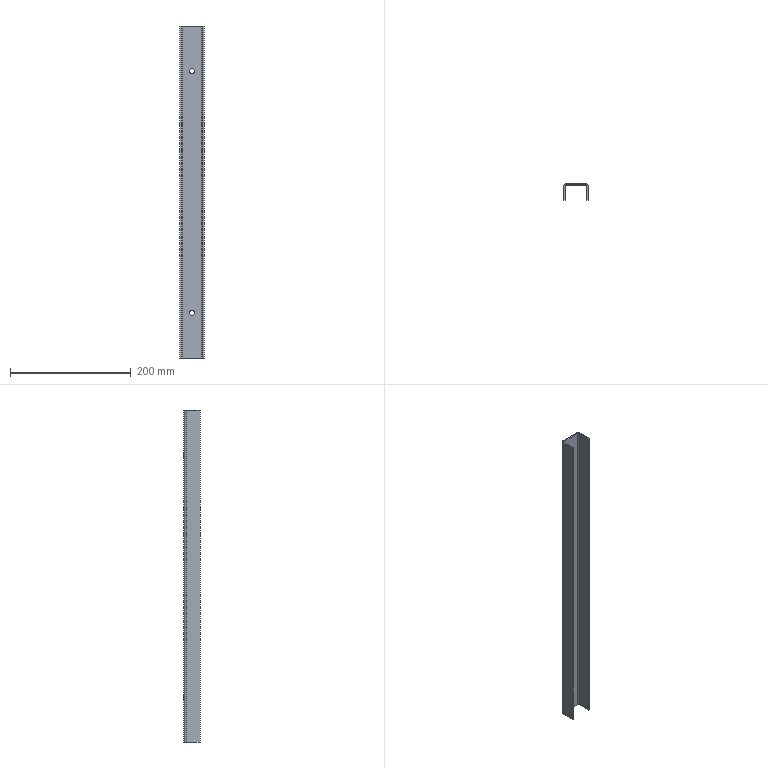Part | STEP file | SYL_0392D6J1SYL0380DJ10-1718718 | 1 solid | 26 faces | box 40 x 27 x 550 mm | volume 95966 mm3 | plane 18 | cylinder 8 | commonest cylinder face diameters 8 x6 4 x2
STEP:
#1=CARTESIAN_POINT('',(0.,14.5,196.));
#2=VERTEX_POINT('',#1);
#3=CARTESIAN_POINT('',(0.,12.5,196.));
#4=VERTEX_POINT('',#3);
#5=CARTESIAN_POINT('',(0.,12.5,196.));
#6=DIRECTION('',(0.,-1.,0.));
#7=VECTOR('',#6,1000.);
#8=LINE('',#5,#7);
#9=EDGE_CURVE('',#2,#4,#8,.T.);
#10=ORIENTED_EDGE('',*,*,#9,.F.);
#11=CARTESIAN_POINT('',(0.,14.5,204.));
#12=VERTEX_POINT('',#11);
#13=CARTESIAN_POINT('',(0.,14.5,200.));
#14=DIRECTION('',(0.,1.,0.));
#15=DIRECTION('',(0.,0.,1.));
#16=AXIS2_PLACEMENT_3D('',#13,#14,#15);
#17=CIRCLE('',#16,4.);
#18=EDGE_CURVE('',#2,#12,#17,.T.);
#19=ORIENTED_EDGE('',*,*,#18,.T.);
#20=CARTESIAN_POINT('',(0.,12.5,204.));
#21=VERTEX_POINT('',#20);
#22=CARTESIAN_POINT('',(0.,12.5,204.));
#23=DIRECTION('',(0.,-1.,0.));
#24=VECTOR('',#23,1000.);
#25=LINE('',#22,#24);
#26=EDGE_CURVE('',#12,#21,#25,.T.);
#27=ORIENTED_EDGE('',*,*,#26,.T.);
#28=CARTESIAN_POINT('',(0.,12.5,200.));
#29=DIRECTION('',(0.,1.,0.));
#30=DIRECTION('',(0.,0.,-1.));
#31=AXIS2_PLACEMENT_3D('',#28,#29,#30);
#32=CIRCLE('',#31,4.);
#33=EDGE_CURVE('',#4,#21,#32,.T.);
#34=ORIENTED_EDGE('',*,*,#33,.F.);
#35=EDGE_LOOP('',(#10,#19,#27,#34));
#36=FACE_OUTER_BOUND('',#35,.T.);
#37=CARTESIAN_POINT('',(0.,12.5,200.));
#38=DIRECTION('',(0.,-1.,0.));
#39=DIRECTION('',(0.,0.,-1.));
#40=AXIS2_PLACEMENT_3D('',#37,#38,#39);
#41=CYLINDRICAL_SURFACE('',#40,4.);
#42=ADVANCED_FACE('',(#36),#41,.F.);
#43=CARTESIAN_POINT('',(0.,14.5,-204.));
#44=VERTEX_POINT('',#43);
#45=CARTESIAN_POINT('',(0.,12.5,-204.));
#46=VERTEX_POINT('',#45);
#47=CARTESIAN_POINT('',(0.,12.5,-204.));
#48=DIRECTION('',(0.,-1.,0.));
#49=VECTOR('',#48,1000.);
#50=LINE('',#47,#49);
#51=EDGE_CURVE('',#44,#46,#50,.T.);
#52=ORIENTED_EDGE('',*,*,#51,.F.);
#53=CARTESIAN_POINT('',(0.,14.5,-196.));
#54=VERTEX_POINT('',#53);
#55=CARTESIAN_POINT('',(0.,14.5,-200.));
#56=DIRECTION('',(0.,1.,0.));
#57=DIRECTION('',(0.,0.,1.));
#58=AXIS2_PLACEMENT_3D('',#55,#56,#57);
#59=CIRCLE('',#58,4.);
#60=EDGE_CURVE('',#44,#54,#59,.T.);
#61=ORIENTED_EDGE('',*,*,#60,.T.);
#62=CARTESIAN_POINT('',(0.,12.5,-196.));
#63=VERTEX_POINT('',#62);
#64=CARTESIAN_POINT('',(0.,12.5,-196.));
#65=DIRECTION('',(0.,-1.,0.));
#66=VECTOR('',#65,1000.);
#67=LINE('',#64,#66);
#68=EDGE_CURVE('',#54,#63,#67,.T.);
#69=ORIENTED_EDGE('',*,*,#68,.T.);
#70=CARTESIAN_POINT('',(0.,12.5,-200.));
#71=DIRECTION('',(0.,1.,0.));
#72=DIRECTION('',(0.,0.,-1.));
#73=AXIS2_PLACEMENT_3D('',#70,#71,#72);
#74=CIRCLE('',#73,4.);
#75=EDGE_CURVE('',#46,#63,#74,.T.);
#76=ORIENTED_EDGE('',*,*,#75,.F.);
#77=EDGE_LOOP('',(#52,#61,#69,#76));
#78=FACE_OUTER_BOUND('',#77,.T.);
#79=CARTESIAN_POINT('',(0.,12.5,-200.));
#80=DIRECTION('',(0.,-1.,0.));
#81=DIRECTION('',(0.,0.,-1.));
#82=AXIS2_PLACEMENT_3D('',#79,#80,#81);
#83=CYLINDRICAL_SURFACE('',#82,4.);
#84=ADVANCED_FACE('',(#78),#83,.F.);
#85=CARTESIAN_POINT('',(16.,14.5,-275.));
#86=VERTEX_POINT('',#85);
#87=CARTESIAN_POINT('',(16.,12.5,-275.));
#88=VERTEX_POINT('',#87);
#89=CARTESIAN_POINT('',(16.,12.5,-275.));
#90=DIRECTION('',(0.,-1.,0.));
#91=VECTOR('',#90,1000.);
#92=LINE('',#89,#91);
#93=EDGE_CURVE('',#86,#88,#92,.T.);
#94=ORIENTED_EDGE('',*,*,#93,.F.);
#95=CARTESIAN_POINT('',(20.,10.5,-275.));
#96=VERTEX_POINT('',#95);
#97=CARTESIAN_POINT('',(16.,10.5,-275.));
#98=DIRECTION('',(0.,0.,1.));
#99=DIRECTION('',(1.,0.,0.));
#100=AXIS2_PLACEMENT_3D('',#97,#98,#99);
#101=CIRCLE('',#100,4.);
#102=EDGE_CURVE('',#96,#86,#101,.T.);
#103=ORIENTED_EDGE('',*,*,#102,.F.);
#104=CARTESIAN_POINT('',(18.,10.5,-275.));
#105=VERTEX_POINT('',#104);
#106=CARTESIAN_POINT('',(18.,10.5,-275.));
#107=DIRECTION('',(-1.,0.,0.));
#108=VECTOR('',#107,1000.);
#109=LINE('',#106,#108);
#110=EDGE_CURVE('',#96,#105,#109,.T.);
#111=ORIENTED_EDGE('',*,*,#110,.T.);
#112=CARTESIAN_POINT('',(16.,10.5,-275.));
#113=DIRECTION('',(0.,0.,1.));
#114=DIRECTION('',(1.,0.,0.));
#115=AXIS2_PLACEMENT_3D('',#112,#113,#114);
#116=CIRCLE('',#115,2.);
#117=EDGE_CURVE('',#105,#88,#116,.T.);
#118=ORIENTED_EDGE('',*,*,#117,.T.);
#119=EDGE_LOOP('',(#94,#103,#111,#118));
#120=FACE_OUTER_BOUND('',#119,.T.);
#121=CARTESIAN_POINT('',(16.,10.5,-275.));
#122=DIRECTION('',(0.,0.,-1.));
#123=DIRECTION('',(-1.,0.,0.));
#124=AXIS2_PLACEMENT_3D('',#121,#122,#123);
#125=PLANE('',#124);
#126=ADVANCED_FACE('',(#120),#125,.T.);
#127=ORIENTED_EDGE('',*,*,#110,.F.);
#128=CARTESIAN_POINT('',(20.,-12.5,-275.));
#129=VERTEX_POINT('',#128);
#130=CARTESIAN_POINT('',(20.,12.5,-275.));
#131=DIRECTION('',(0.,-1.,0.));
#132=VECTOR('',#131,1000.);
#133=LINE('',#130,#132);
#134=EDGE_CURVE('',#96,#129,#133,.T.);
#135=ORIENTED_EDGE('',*,*,#134,.T.);
#136=CARTESIAN_POINT('',(18.,-12.5,-275.));
#137=VERTEX_POINT('',#136);
#138=CARTESIAN_POINT('',(18.,-12.5,-275.));
#139=DIRECTION('',(-1.,0.,0.));
#140=VECTOR('',#139,1000.);
#141=LINE('',#138,#140);
#142=EDGE_CURVE('',#129,#137,#141,.T.);
#143=ORIENTED_EDGE('',*,*,#142,.T.);
#144=CARTESIAN_POINT('',(18.,10.5,-275.));
#145=DIRECTION('',(0.,-1.,0.));
#146=VECTOR('',#145,1000.);
#147=LINE('',#144,#146);
#148=EDGE_CURVE('',#105,#137,#147,.T.);
#149=ORIENTED_EDGE('',*,*,#148,.F.);
#150=EDGE_LOOP('',(#127,#135,#143,#149));
#151=FACE_OUTER_BOUND('',#150,.T.);
#152=CARTESIAN_POINT('',(18.,10.5,-275.));
#153=DIRECTION('',(0.,0.,-1.));
#154=DIRECTION('',(0.,-1.,0.));
#155=AXIS2_PLACEMENT_3D('',#152,#153,#154);
#156=PLANE('',#155);
#157=ADVANCED_FACE('',(#151),#156,.T.);
#158=ORIENTED_EDGE('',*,*,#142,.F.);
#159=CARTESIAN_POINT('',(20.,-12.5,275.));
#160=VERTEX_POINT('',#159);
#161=CARTESIAN_POINT('',(20.,-12.5,-275.));
#162=DIRECTION('',(0.,0.,1.));
#163=VECTOR('',#162,1000.);
#164=LINE('',#161,#163);
#165=EDGE_CURVE('',#129,#160,#164,.T.);
#166=ORIENTED_EDGE('',*,*,#165,.T.);
#167=CARTESIAN_POINT('',(18.,-12.5,275.));
#168=VERTEX_POINT('',#167);
#169=CARTESIAN_POINT('',(18.,-12.5,275.));
#170=DIRECTION('',(-1.,0.,0.));
#171=VECTOR('',#170,1000.);
#172=LINE('',#169,#171);
#173=EDGE_CURVE('',#160,#168,#172,.T.);
#174=ORIENTED_EDGE('',*,*,#173,.T.);
#175=CARTESIAN_POINT('',(18.,-12.5,-275.));
#176=DIRECTION('',(0.,0.,1.));
#177=VECTOR('',#176,1000.);
#178=LINE('',#175,#177);
#179=EDGE_CURVE('',#137,#168,#178,.T.);
#180=ORIENTED_EDGE('',*,*,#179,.F.);
#181=EDGE_LOOP('',(#158,#166,#174,#180));
#182=FACE_OUTER_BOUND('',#181,.T.);
#183=CARTESIAN_POINT('',(18.,-12.5,-275.));
#184=DIRECTION('',(0.,-1.,0.));
#185=DIRECTION('',(0.,0.,1.));
#186=AXIS2_PLACEMENT_3D('',#183,#184,#185);
#187=PLANE('',#186);
#188=ADVANCED_FACE('',(#182),#187,.T.);
#189=ORIENTED_EDGE('',*,*,#173,.F.);
#190=CARTESIAN_POINT('',(20.,10.5,275.));
#191=VERTEX_POINT('',#190);
#192=CARTESIAN_POINT('',(20.,12.5,275.));
#193=DIRECTION('',(0.,-1.,0.));
#194=VECTOR('',#193,1000.);
#195=LINE('',#192,#194);
#196=EDGE_CURVE('',#191,#160,#195,.T.);
#197=ORIENTED_EDGE('',*,*,#196,.F.);
#198=CARTESIAN_POINT('',(18.,10.5,275.));
#199=VERTEX_POINT('',#198);
#200=CARTESIAN_POINT('',(18.,10.5,275.));
#201=DIRECTION('',(-1.,0.,0.));
#202=VECTOR('',#201,1000.);
#203=LINE('',#200,#202);
#204=EDGE_CURVE('',#191,#199,#203,.T.);
#205=ORIENTED_EDGE('',*,*,#204,.T.);
#206=CARTESIAN_POINT('',(18.,10.5,275.));
#207=DIRECTION('',(0.,-1.,0.));
#208=VECTOR('',#207,1000.);
#209=LINE('',#206,#208);
#210=EDGE_CURVE('',#199,#168,#209,.T.);
#211=ORIENTED_EDGE('',*,*,#210,.T.);
#212=EDGE_LOOP('',(#189,#197,#205,#211));
#213=FACE_OUTER_BOUND('',#212,.T.);
#214=CARTESIAN_POINT('',(18.,10.5,275.));
#215=DIRECTION('',(0.,0.,-1.));
#216=DIRECTION('',(0.,-1.,0.));
#217=AXIS2_PLACEMENT_3D('',#214,#215,#216);
#218=PLANE('',#217);
#219=ADVANCED_FACE('',(#213),#218,.F.);
#220=ORIENTED_EDGE('',*,*,#204,.F.);
#221=CARTESIAN_POINT('',(16.,14.5,275.));
#222=VERTEX_POINT('',#221);
#223=CARTESIAN_POINT('',(16.,10.5,275.));
#224=DIRECTION('',(0.,0.,-1.));
#225=DIRECTION('',(1.,0.,0.));
#226=AXIS2_PLACEMENT_3D('',#223,#224,#225);
#227=CIRCLE('',#226,4.);
#228=EDGE_CURVE('',#222,#191,#227,.T.);
#229=ORIENTED_EDGE('',*,*,#228,.F.);
#230=CARTESIAN_POINT('',(16.,12.5,275.));
#231=VERTEX_POINT('',#230);
#232=CARTESIAN_POINT('',(16.,12.5,275.));
#233=DIRECTION('',(0.,-1.,0.));
#234=VECTOR('',#233,1000.);
#235=LINE('',#232,#234);
#236=EDGE_CURVE('',#222,#231,#235,.T.);
#237=ORIENTED_EDGE('',*,*,#236,.T.);
#238=CARTESIAN_POINT('',(16.,10.5,275.));
#239=DIRECTION('',(0.,0.,-1.));
#240=DIRECTION('',(0.,1.,0.));
#241=AXIS2_PLACEMENT_3D('',#238,#239,#240);
#242=CIRCLE('',#241,2.);
#243=EDGE_CURVE('',#231,#199,#242,.T.);
#244=ORIENTED_EDGE('',*,*,#243,.T.);
#245=EDGE_LOOP('',(#220,#229,#237,#244));
#246=FACE_OUTER_BOUND('',#245,.T.);
#247=CARTESIAN_POINT('',(16.,10.5,275.));
#248=DIRECTION('',(0.,0.,1.));
#249=DIRECTION('',(1.,0.,0.));
#250=AXIS2_PLACEMENT_3D('',#247,#248,#249);
#251=PLANE('',#250);
#252=ADVANCED_FACE('',(#246),#251,.T.);
#253=ORIENTED_EDGE('',*,*,#236,.F.);
#254=CARTESIAN_POINT('',(-16.,14.5,275.));
#255=VERTEX_POINT('',#254);
#256=CARTESIAN_POINT('',(-18.,14.5,275.));
#257=DIRECTION('',(1.,0.,0.));
#258=VECTOR('',#257,1000.);
#259=LINE('',#256,#258);
#260=EDGE_CURVE('',#255,#222,#259,.T.);
#261=ORIENTED_EDGE('',*,*,#260,.F.);
#262=CARTESIAN_POINT('',(-16.,12.5,275.));
#263=VERTEX_POINT('',#262);
#264=CARTESIAN_POINT('',(-16.,12.5,275.));
#265=DIRECTION('',(0.,-1.,0.));
#266=VECTOR('',#265,1000.);
#267=LINE('',#264,#266);
#268=EDGE_CURVE('',#255,#263,#267,.T.);
#269=ORIENTED_EDGE('',*,*,#268,.T.);
#270=CARTESIAN_POINT('',(-16.,12.5,275.));
#271=DIRECTION('',(1.,0.,0.));
#272=VECTOR('',#271,1000.);
#273=LINE('',#270,#272);
#274=EDGE_CURVE('',#263,#231,#273,.T.);
#275=ORIENTED_EDGE('',*,*,#274,.T.);
#276=EDGE_LOOP('',(#253,#261,#269,#275));
#277=FACE_OUTER_BOUND('',#276,.T.);
#278=CARTESIAN_POINT('',(-16.,12.5,275.));
#279=DIRECTION('',(0.,0.,-1.));
#280=DIRECTION('',(1.,0.,0.));
#281=AXIS2_PLACEMENT_3D('',#278,#279,#280);
#282=PLANE('',#281);
#283=ADVANCED_FACE('',(#277),#282,.F.);
#284=ORIENTED_EDGE('',*,*,#268,.F.);
#285=CARTESIAN_POINT('',(-20.,10.5,275.));
#286=VERTEX_POINT('',#285);
#287=CARTESIAN_POINT('',(-16.,10.5,275.));
#288=DIRECTION('',(0.,0.,-1.));
#289=DIRECTION('',(1.,0.,0.));
#290=AXIS2_PLACEMENT_3D('',#287,#288,#289);
#291=CIRCLE('',#290,4.);
#292=EDGE_CURVE('',#286,#255,#291,.T.);
#293=ORIENTED_EDGE('',*,*,#292,.F.);
#294=CARTESIAN_POINT('',(-18.,10.5,275.));
#295=VERTEX_POINT('',#294);
#296=CARTESIAN_POINT('',(-18.,10.5,275.));
#297=DIRECTION('',(1.,0.,0.));
#298=VECTOR('',#297,1000.);
#299=LINE('',#296,#298);
#300=EDGE_CURVE('',#286,#295,#299,.T.);
#301=ORIENTED_EDGE('',*,*,#300,.T.);
#302=CARTESIAN_POINT('',(-16.,10.5,275.));
#303=DIRECTION('',(0.,0.,-1.));
#304=DIRECTION('',(-1.,0.,0.));
#305=AXIS2_PLACEMENT_3D('',#302,#303,#304);
#306=CIRCLE('',#305,2.);
#307=EDGE_CURVE('',#295,#263,#306,.T.);
#308=ORIENTED_EDGE('',*,*,#307,.T.);
#309=EDGE_LOOP('',(#284,#293,#301,#308));
#310=FACE_OUTER_BOUND('',#309,.T.);
#311=CARTESIAN_POINT('',(-16.,10.5,275.));
#312=DIRECTION('',(0.,0.,1.));
#313=DIRECTION('',(1.,0.,0.));
#314=AXIS2_PLACEMENT_3D('',#311,#312,#313);
#315=PLANE('',#314);
#316=ADVANCED_FACE('',(#310),#315,.T.);
#317=ORIENTED_EDGE('',*,*,#300,.F.);
#318=CARTESIAN_POINT('',(-20.,-12.5,275.));
#319=VERTEX_POINT('',#318);
#320=CARTESIAN_POINT('',(-20.,-12.5,275.));
#321=DIRECTION('',(0.,1.,0.));
#322=VECTOR('',#321,1000.);
#323=LINE('',#320,#322);
#324=EDGE_CURVE('',#319,#286,#323,.T.);
#325=ORIENTED_EDGE('',*,*,#324,.F.);
#326=CARTESIAN_POINT('',(-18.,-12.5,275.));
#327=VERTEX_POINT('',#326);
#328=CARTESIAN_POINT('',(-18.,-12.5,275.));
#329=DIRECTION('',(1.,0.,0.));
#330=VECTOR('',#329,1000.);
#331=LINE('',#328,#330);
#332=EDGE_CURVE('',#319,#327,#331,.T.);
#333=ORIENTED_EDGE('',*,*,#332,.T.);
#334=CARTESIAN_POINT('',(-18.,-12.5,275.));
#335=DIRECTION('',(0.,1.,0.));
#336=VECTOR('',#335,1000.);
#337=LINE('',#334,#336);
#338=EDGE_CURVE('',#327,#295,#337,.T.);
#339=ORIENTED_EDGE('',*,*,#338,.T.);
#340=EDGE_LOOP('',(#317,#325,#333,#339));
#341=FACE_OUTER_BOUND('',#340,.T.);
#342=CARTESIAN_POINT('',(-18.,-12.5,275.));
#343=DIRECTION('',(0.,0.,-1.));
#344=DIRECTION('',(0.,1.,0.));
#345=AXIS2_PLACEMENT_3D('',#342,#343,#344);
#346=PLANE('',#345);
#347=ADVANCED_FACE('',(#341),#346,.F.);
#348=ORIENTED_EDGE('',*,*,#332,.F.);
#349=CARTESIAN_POINT('',(-20.,-12.5,-275.));
#350=VERTEX_POINT('',#349);
#351=CARTESIAN_POINT('',(-20.,-12.5,-275.));
#352=DIRECTION('',(0.,0.,1.));
#353=VECTOR('',#352,1000.);
#354=LINE('',#351,#353);
#355=EDGE_CURVE('',#350,#319,#354,.T.);
#356=ORIENTED_EDGE('',*,*,#355,.F.);
#357=CARTESIAN_POINT('',(-18.,-12.5,-275.));
#358=VERTEX_POINT('',#357);
#359=CARTESIAN_POINT('',(-18.,-12.5,-275.));
#360=DIRECTION('',(1.,0.,0.));
#361=VECTOR('',#360,1000.);
#362=LINE('',#359,#361);
#363=EDGE_CURVE('',#350,#358,#362,.T.);
#364=ORIENTED_EDGE('',*,*,#363,.T.);
#365=CARTESIAN_POINT('',(-18.,-12.5,-275.));
#366=DIRECTION('',(0.,0.,1.));
#367=VECTOR('',#366,1000.);
#368=LINE('',#365,#367);
#369=EDGE_CURVE('',#358,#327,#368,.T.);
#370=ORIENTED_EDGE('',*,*,#369,.T.);
#371=EDGE_LOOP('',(#348,#356,#364,#370));
#372=FACE_OUTER_BOUND('',#371,.T.);
#373=CARTESIAN_POINT('',(-18.,-12.5,-275.));
#374=DIRECTION('',(0.,1.,0.));
#375=DIRECTION('',(0.,0.,1.));
#376=AXIS2_PLACEMENT_3D('',#373,#374,#375);
#377=PLANE('',#376);
#378=ADVANCED_FACE('',(#372),#377,.F.);
#379=ORIENTED_EDGE('',*,*,#363,.F.);
#380=CARTESIAN_POINT('',(-20.,10.5,-275.));
#381=VERTEX_POINT('',#380);
#382=CARTESIAN_POINT('',(-20.,-12.5,-275.));
#383=DIRECTION('',(0.,1.,0.));
#384=VECTOR('',#383,1000.);
#385=LINE('',#382,#384);
#386=EDGE_CURVE('',#350,#381,#385,.T.);
#387=ORIENTED_EDGE('',*,*,#386,.T.);
#388=CARTESIAN_POINT('',(-18.,10.5,-275.));
#389=VERTEX_POINT('',#388);
#390=CARTESIAN_POINT('',(-18.,10.5,-275.));
#391=DIRECTION('',(1.,0.,0.));
#392=VECTOR('',#391,1000.);
#393=LINE('',#390,#392);
#394=EDGE_CURVE('',#381,#389,#393,.T.);
#395=ORIENTED_EDGE('',*,*,#394,.T.);
#396=CARTESIAN_POINT('',(-18.,-12.5,-275.));
#397=DIRECTION('',(0.,1.,0.));
#398=VECTOR('',#397,1000.);
#399=LINE('',#396,#398);
#400=EDGE_CURVE('',#358,#389,#399,.T.);
#401=ORIENTED_EDGE('',*,*,#400,.F.);
#402=EDGE_LOOP('',(#379,#387,#395,#401));
#403=FACE_OUTER_BOUND('',#402,.T.);
#404=CARTESIAN_POINT('',(-18.,-12.5,-275.));
#405=DIRECTION('',(0.,0.,-1.));
#406=DIRECTION('',(0.,1.,0.));
#407=AXIS2_PLACEMENT_3D('',#404,#405,#406);
#408=PLANE('',#407);
#409=ADVANCED_FACE('',(#403),#408,.T.);
#410=ORIENTED_EDGE('',*,*,#394,.F.);
#411=CARTESIAN_POINT('',(-16.,14.5,-275.));
#412=VERTEX_POINT('',#411);
#413=CARTESIAN_POINT('',(-16.,10.5,-275.));
#414=DIRECTION('',(0.,0.,1.));
#415=DIRECTION('',(1.,0.,0.));
#416=AXIS2_PLACEMENT_3D('',#413,#414,#415);
#417=CIRCLE('',#416,4.);
#418=EDGE_CURVE('',#412,#381,#417,.T.);
#419=ORIENTED_EDGE('',*,*,#418,.F.);
#420=CARTESIAN_POINT('',(-16.,12.5,-275.));
#421=VERTEX_POINT('',#420);
#422=CARTESIAN_POINT('',(-16.,12.5,-275.));
#423=DIRECTION('',(0.,-1.,0.));
#424=VECTOR('',#423,1000.);
#425=LINE('',#422,#424);
#426=EDGE_CURVE('',#412,#421,#425,.T.);
#427=ORIENTED_EDGE('',*,*,#426,.T.);
#428=CARTESIAN_POINT('',(-16.,10.5,-275.));
#429=DIRECTION('',(0.,0.,1.));
#430=DIRECTION('',(0.,1.,0.));
#431=AXIS2_PLACEMENT_3D('',#428,#429,#430);
#432=CIRCLE('',#431,2.);
#433=EDGE_CURVE('',#421,#389,#432,.T.);
#434=ORIENTED_EDGE('',*,*,#433,.T.);
#435=EDGE_LOOP('',(#410,#419,#427,#434));
#436=FACE_OUTER_BOUND('',#435,.T.);
#437=CARTESIAN_POINT('',(-16.,10.5,-275.));
#438=DIRECTION('',(0.,0.,-1.));
#439=DIRECTION('',(-1.,0.,0.));
#440=AXIS2_PLACEMENT_3D('',#437,#438,#439);
#441=PLANE('',#440);
#442=ADVANCED_FACE('',(#436),#441,.T.);
#443=CARTESIAN_POINT('',(0.,14.5,-200.));
#444=DIRECTION('',(0.,1.,0.));
#445=DIRECTION('',(0.,0.,1.));
#446=AXIS2_PLACEMENT_3D('',#443,#444,#445);
#447=CIRCLE('',#446,4.);
#448=EDGE_CURVE('',#54,#44,#447,.T.);
#449=ORIENTED_EDGE('',*,*,#448,.T.);
#450=ORIENTED_EDGE('',*,*,#51,.T.);
#451=CARTESIAN_POINT('',(0.,12.5,-200.));
#452=DIRECTION('',(0.,1.,0.));
#453=DIRECTION('',(0.,0.,1.));
#454=AXIS2_PLACEMENT_3D('',#451,#452,#453);
#455=CIRCLE('',#454,4.);
#456=EDGE_CURVE('',#63,#46,#455,.T.);
#457=ORIENTED_EDGE('',*,*,#456,.F.);
#458=ORIENTED_EDGE('',*,*,#68,.F.);
#459=EDGE_LOOP('',(#449,#450,#457,#458));
#460=FACE_OUTER_BOUND('',#459,.T.);
#461=CARTESIAN_POINT('',(0.,12.5,-200.));
#462=DIRECTION('',(0.,-1.,0.));
#463=DIRECTION('',(0.,0.,-1.));
#464=AXIS2_PLACEMENT_3D('',#461,#462,#463);
#465=CYLINDRICAL_SURFACE('',#464,4.);
#466=ADVANCED_FACE('',(#460),#465,.F.);
#467=CARTESIAN_POINT('',(0.,14.5,200.));
#468=DIRECTION('',(0.,1.,0.));
#469=DIRECTION('',(0.,0.,1.));
#470=AXIS2_PLACEMENT_3D('',#467,#468,#469);
#471=CIRCLE('',#470,4.);
#472=EDGE_CURVE('',#12,#2,#471,.T.);
#473=ORIENTED_EDGE('',*,*,#472,.T.);
#474=ORIENTED_EDGE('',*,*,#9,.T.);
#475=CARTESIAN_POINT('',(0.,12.5,200.));
#476=DIRECTION('',(0.,1.,0.));
#477=DIRECTION('',(0.,0.,1.));
#478=AXIS2_PLACEMENT_3D('',#475,#476,#477);
#479=CIRCLE('',#478,4.);
#480=EDGE_CURVE('',#21,#4,#479,.T.);
#481=ORIENTED_EDGE('',*,*,#480,.F.);
#482=ORIENTED_EDGE('',*,*,#26,.F.);
#483=EDGE_LOOP('',(#473,#474,#481,#482));
#484=FACE_OUTER_BOUND('',#483,.T.);
#485=CARTESIAN_POINT('',(0.,12.5,200.));
#486=DIRECTION('',(0.,-1.,0.));
#487=DIRECTION('',(0.,0.,-1.));
#488=AXIS2_PLACEMENT_3D('',#485,#486,#487);
#489=CYLINDRICAL_SURFACE('',#488,4.);
#490=ADVANCED_FACE('',(#484),#489,.F.);
#491=CARTESIAN_POINT('',(-18.,14.5,-275.));
#492=DIRECTION('',(1.,0.,0.));
#493=VECTOR('',#492,1000.);
#494=LINE('',#491,#493);
#495=EDGE_CURVE('',#412,#86,#494,.T.);
#496=ORIENTED_EDGE('',*,*,#495,.T.);
#497=ORIENTED_EDGE('',*,*,#93,.T.);
#498=CARTESIAN_POINT('',(-16.,12.5,-275.));
#499=DIRECTION('',(1.,0.,0.));
#500=VECTOR('',#499,1000.);
#501=LINE('',#498,#500);
#502=EDGE_CURVE('',#421,#88,#501,.T.);
#503=ORIENTED_EDGE('',*,*,#502,.F.);
#504=ORIENTED_EDGE('',*,*,#426,.F.);
#505=EDGE_LOOP('',(#496,#497,#503,#504));
#506=FACE_OUTER_BOUND('',#505,.T.);
#507=CARTESIAN_POINT('',(-16.,12.5,-275.));
#508=DIRECTION('',(0.,0.,-1.));
#509=DIRECTION('',(1.,0.,0.));
#510=AXIS2_PLACEMENT_3D('',#507,#508,#509);
#511=PLANE('',#510);
#512=ADVANCED_FACE('',(#506),#511,.T.);
#513=ORIENTED_EDGE('',*,*,#433,.F.);
#514=CARTESIAN_POINT('',(-16.,12.5,-275.));
#515=DIRECTION('',(0.,0.,1.));
#516=VECTOR('',#515,1000.);
#517=LINE('',#514,#516);
#518=EDGE_CURVE('',#421,#263,#517,.T.);
#519=ORIENTED_EDGE('',*,*,#518,.T.);
#520=ORIENTED_EDGE('',*,*,#307,.F.);
#521=CARTESIAN_POINT('',(-18.,10.5,275.));
#522=DIRECTION('',(0.,0.,-1.));
#523=VECTOR('',#522,1000.);
#524=LINE('',#521,#523);
#525=EDGE_CURVE('',#295,#389,#524,.T.);
#526=ORIENTED_EDGE('',*,*,#525,.T.);
#527=EDGE_LOOP('',(#513,#519,#520,#526));
#528=FACE_OUTER_BOUND('',#527,.T.);
#529=CARTESIAN_POINT('',(-16.,10.5,-275.));
#530=DIRECTION('',(0.,0.,1.));
#531=DIRECTION('',(1.,0.,0.));
#532=AXIS2_PLACEMENT_3D('',#529,#530,#531);
#533=CYLINDRICAL_SURFACE('',#532,2.);
#534=ADVANCED_FACE('',(#528),#533,.F.);
#535=ORIENTED_EDGE('',*,*,#400,.T.);
#536=ORIENTED_EDGE('',*,*,#525,.F.);
#537=ORIENTED_EDGE('',*,*,#338,.F.);
#538=ORIENTED_EDGE('',*,*,#369,.F.);
#539=EDGE_LOOP('',(#535,#536,#537,#538));
#540=FACE_OUTER_BOUND('',#539,.T.);
#541=CARTESIAN_POINT('',(-18.,-12.5,-275.));
#542=DIRECTION('',(1.,0.,0.));
#543=DIRECTION('',(0.,1.,0.));
#544=AXIS2_PLACEMENT_3D('',#541,#542,#543);
#545=PLANE('',#544);
#546=ADVANCED_FACE('',(#540),#545,.T.);
#547=ORIENTED_EDGE('',*,*,#117,.F.);
#548=CARTESIAN_POINT('',(18.,10.5,-275.));
#549=DIRECTION('',(0.,0.,1.));
#550=VECTOR('',#549,1000.);
#551=LINE('',#548,#550);
#552=EDGE_CURVE('',#105,#199,#551,.T.);
#553=ORIENTED_EDGE('',*,*,#552,.T.);
#554=ORIENTED_EDGE('',*,*,#243,.F.);
#555=CARTESIAN_POINT('',(16.,12.5,275.));
#556=DIRECTION('',(0.,0.,-1.));
#557=VECTOR('',#556,1000.);
#558=LINE('',#555,#557);
#559=EDGE_CURVE('',#231,#88,#558,.T.);
#560=ORIENTED_EDGE('',*,*,#559,.T.);
#561=EDGE_LOOP('',(#547,#553,#554,#560));
#562=FACE_OUTER_BOUND('',#561,.T.);
#563=CARTESIAN_POINT('',(16.,10.5,-275.));
#564=DIRECTION('',(0.,0.,1.));
#565=DIRECTION('',(1.,0.,0.));
#566=AXIS2_PLACEMENT_3D('',#563,#564,#565);
#567=CYLINDRICAL_SURFACE('',#566,2.);
#568=ADVANCED_FACE('',(#562),#567,.F.);
#569=ORIENTED_EDGE('',*,*,#75,.T.);
#570=ORIENTED_EDGE('',*,*,#456,.T.);
#571=EDGE_LOOP('',(#569,#570));
#572=FACE_BOUND('',#571,.T.);
#573=ORIENTED_EDGE('',*,*,#33,.T.);
#574=ORIENTED_EDGE('',*,*,#480,.T.);
#575=EDGE_LOOP('',(#573,#574));
#576=FACE_BOUND('',#575,.T.);
#577=ORIENTED_EDGE('',*,*,#502,.T.);
#578=ORIENTED_EDGE('',*,*,#559,.F.);
#579=ORIENTED_EDGE('',*,*,#274,.F.);
#580=ORIENTED_EDGE('',*,*,#518,.F.);
#581=EDGE_LOOP('',(#577,#578,#579,#580));
#582=FACE_OUTER_BOUND('',#581,.T.);
#583=CARTESIAN_POINT('',(-18.,12.5,-275.));
#584=DIRECTION('',(0.,-1.,0.));
#585=DIRECTION('',(0.,0.,-1.));
#586=AXIS2_PLACEMENT_3D('',#583,#584,#585);
#587=PLANE('',#586);
#588=ADVANCED_FACE('',(#572,#576,#582),#587,.T.);
#589=ORIENTED_EDGE('',*,*,#148,.T.);
#590=ORIENTED_EDGE('',*,*,#179,.T.);
#591=ORIENTED_EDGE('',*,*,#210,.F.);
#592=ORIENTED_EDGE('',*,*,#552,.F.);
#593=EDGE_LOOP('',(#589,#590,#591,#592));
#594=FACE_OUTER_BOUND('',#593,.T.);
#595=CARTESIAN_POINT('',(18.,12.5,-275.));
#596=DIRECTION('',(-1.,0.,0.));
#597=DIRECTION('',(0.,0.,1.));
#598=AXIS2_PLACEMENT_3D('',#595,#596,#597);
#599=PLANE('',#598);
#600=ADVANCED_FACE('',(#594),#599,.T.);
#601=ORIENTED_EDGE('',*,*,#418,.T.);
#602=CARTESIAN_POINT('',(-20.,10.5,-275.));
#603=DIRECTION('',(0.,0.,-1.));
#604=VECTOR('',#603,1000.);
#605=LINE('',#602,#604);
#606=EDGE_CURVE('',#286,#381,#605,.T.);
#607=ORIENTED_EDGE('',*,*,#606,.F.);
#608=ORIENTED_EDGE('',*,*,#292,.T.);
#609=CARTESIAN_POINT('',(-16.,14.5,-275.));
#610=DIRECTION('',(0.,0.,1.));
#611=VECTOR('',#610,1000.);
#612=LINE('',#609,#611);
#613=EDGE_CURVE('',#412,#255,#612,.T.);
#614=ORIENTED_EDGE('',*,*,#613,.F.);
#615=EDGE_LOOP('',(#601,#607,#608,#614));
#616=FACE_OUTER_BOUND('',#615,.T.);
#617=CARTESIAN_POINT('',(-16.,10.5,-275.));
#618=DIRECTION('',(0.,0.,1.));
#619=DIRECTION('',(1.,0.,0.));
#620=AXIS2_PLACEMENT_3D('',#617,#618,#619);
#621=CYLINDRICAL_SURFACE('',#620,4.);
#622=ADVANCED_FACE('',(#616),#621,.T.);
#623=ORIENTED_EDGE('',*,*,#386,.F.);
#624=ORIENTED_EDGE('',*,*,#355,.T.);
#625=ORIENTED_EDGE('',*,*,#324,.T.);
#626=ORIENTED_EDGE('',*,*,#606,.T.);
#627=EDGE_LOOP('',(#623,#624,#625,#626));
#628=FACE_OUTER_BOUND('',#627,.T.);
#629=CARTESIAN_POINT('',(-20.,-12.5,-275.));
#630=DIRECTION('',(1.,0.,0.));
#631=DIRECTION('',(0.,1.,0.));
#632=AXIS2_PLACEMENT_3D('',#629,#630,#631);
#633=PLANE('',#632);
#634=ADVANCED_FACE('',(#628),#633,.F.);
#635=ORIENTED_EDGE('',*,*,#102,.T.);
#636=CARTESIAN_POINT('',(16.,14.5,-275.));
#637=DIRECTION('',(0.,0.,-1.));
#638=VECTOR('',#637,1000.);
#639=LINE('',#636,#638);
#640=EDGE_CURVE('',#222,#86,#639,.T.);
#641=ORIENTED_EDGE('',*,*,#640,.F.);
#642=ORIENTED_EDGE('',*,*,#228,.T.);
#643=CARTESIAN_POINT('',(20.,10.5,-275.));
#644=DIRECTION('',(0.,0.,1.));
#645=VECTOR('',#644,1000.);
#646=LINE('',#643,#645);
#647=EDGE_CURVE('',#96,#191,#646,.T.);
#648=ORIENTED_EDGE('',*,*,#647,.F.);
#649=EDGE_LOOP('',(#635,#641,#642,#648));
#650=FACE_OUTER_BOUND('',#649,.T.);
#651=CARTESIAN_POINT('',(16.,10.5,-275.));
#652=DIRECTION('',(0.,0.,1.));
#653=DIRECTION('',(1.,0.,0.));
#654=AXIS2_PLACEMENT_3D('',#651,#652,#653);
#655=CYLINDRICAL_SURFACE('',#654,4.);
#656=ADVANCED_FACE('',(#650),#655,.T.);
#657=ORIENTED_EDGE('',*,*,#60,.F.);
#658=ORIENTED_EDGE('',*,*,#448,.F.);
#659=EDGE_LOOP('',(#657,#658));
#660=FACE_BOUND('',#659,.T.);
#661=ORIENTED_EDGE('',*,*,#18,.F.);
#662=ORIENTED_EDGE('',*,*,#472,.F.);
#663=EDGE_LOOP('',(#661,#662));
#664=FACE_BOUND('',#663,.T.);
#665=ORIENTED_EDGE('',*,*,#495,.F.);
#666=ORIENTED_EDGE('',*,*,#613,.T.);
#667=ORIENTED_EDGE('',*,*,#260,.T.);
#668=ORIENTED_EDGE('',*,*,#640,.T.);
#669=EDGE_LOOP('',(#665,#666,#667,#668));
#670=FACE_OUTER_BOUND('',#669,.T.);
#671=CARTESIAN_POINT('',(-18.,14.5,-275.));
#672=DIRECTION('',(0.,-1.,0.));
#673=DIRECTION('',(0.,0.,-1.));
#674=AXIS2_PLACEMENT_3D('',#671,#672,#673);
#675=PLANE('',#674);
#676=ADVANCED_FACE('',(#660,#664,#670),#675,.F.);
#677=ORIENTED_EDGE('',*,*,#134,.F.);
#678=ORIENTED_EDGE('',*,*,#647,.T.);
#679=ORIENTED_EDGE('',*,*,#196,.T.);
#680=ORIENTED_EDGE('',*,*,#165,.F.);
#681=EDGE_LOOP('',(#677,#678,#679,#680));
#682=FACE_OUTER_BOUND('',#681,.T.);
#683=CARTESIAN_POINT('',(20.,12.5,-275.));
#684=DIRECTION('',(-1.,0.,0.));
#685=DIRECTION('',(0.,0.,1.));
#686=AXIS2_PLACEMENT_3D('',#683,#684,#685);
#687=PLANE('',#686);
#688=ADVANCED_FACE('',(#682),#687,.F.);
#689=CLOSED_SHELL('',(#42,#84,#126,#157,#188,#219,#252,#283,#316,#347,#378,#409,#442,#466,#490,#512,#534,#546,#568,#588,#600,#622,#634,#656,#676,#688));
#690=MANIFOLD_SOLID_BREP('',#689);
#691=CARTESIAN_POINT('',(0.,0.,0.));
#692=DIRECTION('',(0.,0.,1.));
#693=DIRECTION('',(1.,0.,0.));
#694=AXIS2_PLACEMENT_3D('',#691,#692,#693);
#695=(LENGTH_UNIT()NAMED_UNIT(*)SI_UNIT(.MILLI.,.METRE.));
#696=UNCERTAINTY_MEASURE_WITH_UNIT(LENGTH_MEASURE(0.00001),#695,'','');
#697=(NAMED_UNIT(*)PLANE_ANGLE_UNIT()SI_UNIT($,.RADIAN.));
#698=(NAMED_UNIT(*)SI_UNIT($,.STERADIAN.)SOLID_ANGLE_UNIT());
#699=(GEOMETRIC_REPRESENTATION_CONTEXT(3)GLOBAL_UNCERTAINTY_ASSIGNED_CONTEXT((#696))GLOBAL_UNIT_ASSIGNED_CONTEXT((#695,#697,#698))REPRESENTATION_CONTEXT('',''));
#700=ADVANCED_BREP_SHAPE_REPRESENTATION('',(#690,#694),#699);